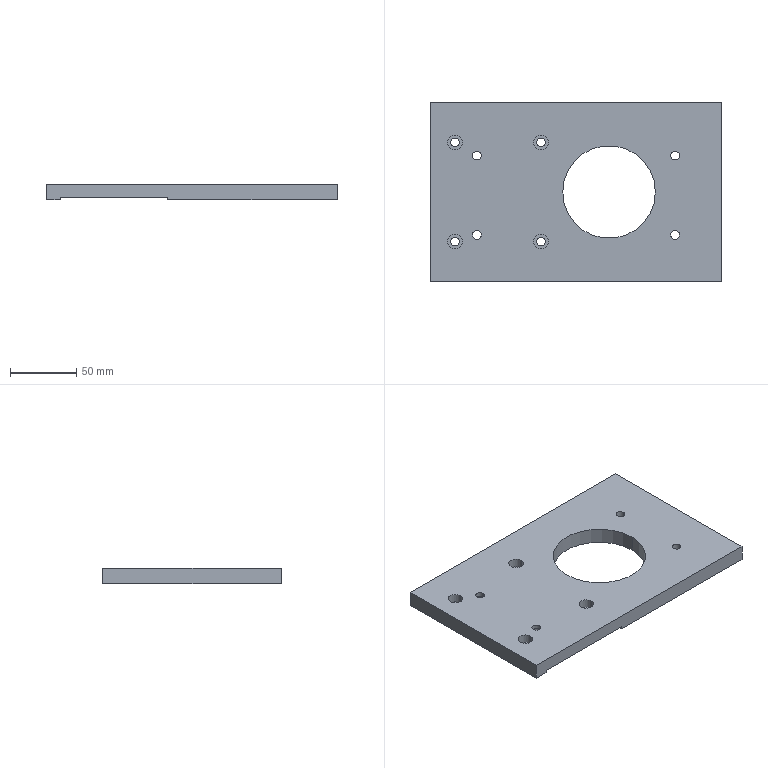Part | SolidWorks | features HoleWzd 4, ICE 2, Extrusion 1 | 1 solid | 64 faces | box 220 x 135 x 12 mm | volume 281633 mm3 | cylinder 40 | plane 18 | cone 6 | commonest cylinder face diameters 6.6 x16 11 x16 4.2 x6 70 x2